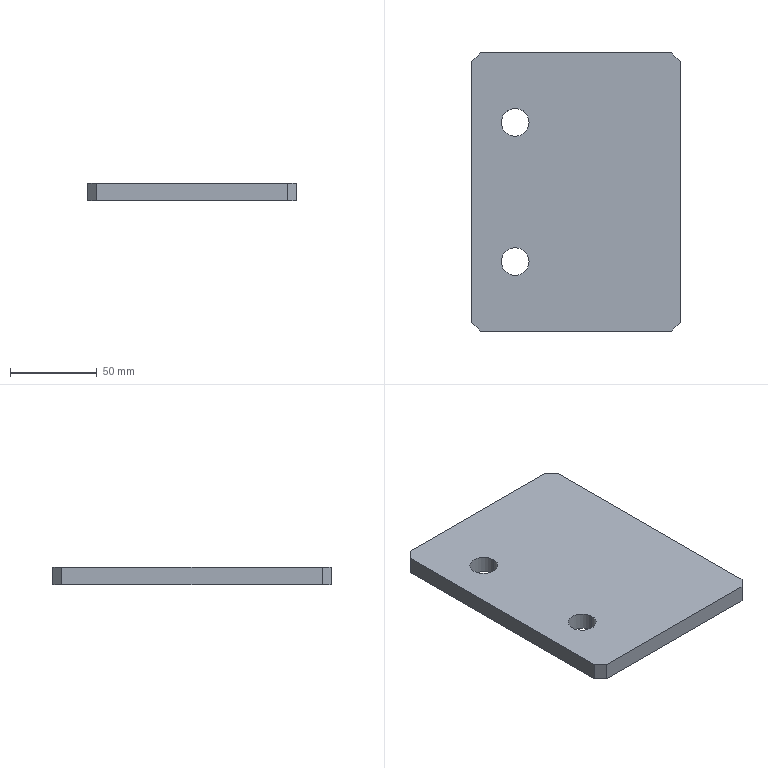Part | STEP file | 中转釜楼梯Pad 1 | 1 solid | 14 faces | box 120 x 160 x 10 mm | volume 187479 mm3 | plane 10 | cylinder 4 | commonest cylinder face diameters 16 x4
STEP:
#1=CARTESIAN_POINT('',(0.,0.,0.));
#2=DIRECTION('',(0.,0.,1.));
#3=DIRECTION('',(1.,0.,0.));
#4=AXIS2_PLACEMENT_3D('',#1,#2,#3);
#5=CARTESIAN_POINT('',(-27.,40.,0.));
#6=VERTEX_POINT('',#5);
#7=CARTESIAN_POINT('',(-27.,40.,10.));
#8=VERTEX_POINT('',#7);
#9=CARTESIAN_POINT('',(-27.,40.,10.));
#10=DIRECTION('',(0.,0.,1.));
#11=VECTOR('',#10,1.);
#12=LINE('',#9,#11);
#13=CARTESIAN_POINT('',(-35.,40.,10.));
#14=DIRECTION('',(0.,0.,1.));
#15=DIRECTION('',(1.,0.,0.));
#16=AXIS2_PLACEMENT_3D('',#13,#14,#15);
#17=CYLINDRICAL_SURFACE('',#16,8.);
#18=CARTESIAN_POINT('',(6.283,0.));
#19=DIRECTION('',(0.,1.));
#20=VECTOR('',#19,1.);
#21=LINE('',#18,#20);
#22=(GEOMETRIC_REPRESENTATION_CONTEXT(2)PARAMETRIC_REPRESENTATION_CONTEXT()REPRESENTATION_CONTEXT('',''));
#23=DEFINITIONAL_REPRESENTATION('',(#21),#22);
#24=PCURVE('',#17,#23);
#25=CARTESIAN_POINT('',(-35.,40.,10.));
#26=DIRECTION('',(0.,0.,1.));
#27=DIRECTION('',(1.,0.,0.));
#28=AXIS2_PLACEMENT_3D('',#25,#26,#27);
#29=CYLINDRICAL_SURFACE('',#28,8.);
#30=CARTESIAN_POINT('',(0.,0.));
#31=DIRECTION('',(0.,1.));
#32=VECTOR('',#31,1.);
#33=LINE('',#30,#32);
#34=(GEOMETRIC_REPRESENTATION_CONTEXT(2)PARAMETRIC_REPRESENTATION_CONTEXT()REPRESENTATION_CONTEXT('',''));
#35=DEFINITIONAL_REPRESENTATION('',(#33),#34);
#36=PCURVE('',#29,#35);
#37=SURFACE_CURVE('',#12,(#24,#36),.PCURVE_S1.);
#38=EDGE_CURVE('',#6,#8,#37,.T.);
#39=ORIENTED_EDGE('',*,*,#38,.T.);
#40=CARTESIAN_POINT('',(-43.,40.,10.));
#41=VERTEX_POINT('',#40);
#42=CARTESIAN_POINT('',(-35.,40.,10.));
#43=DIRECTION('',(0.,0.,1.));
#44=DIRECTION('',(1.,0.,0.));
#45=AXIS2_PLACEMENT_3D('',#42,#43,#44);
#46=CIRCLE('',#45,8.);
#47=CARTESIAN_POINT('',(0.,0.));
#48=DIRECTION('',(1.,0.));
#49=VECTOR('',#48,1.);
#50=LINE('',#47,#49);
#51=(GEOMETRIC_REPRESENTATION_CONTEXT(2)PARAMETRIC_REPRESENTATION_CONTEXT()REPRESENTATION_CONTEXT('',''));
#52=DEFINITIONAL_REPRESENTATION('',(#50),#51);
#53=PCURVE('',#17,#52);
#54=CARTESIAN_POINT('',(0.,0.,10.));
#55=DIRECTION('',(0.,0.,1.));
#56=DIRECTION('',(1.,0.,0.));
#57=AXIS2_PLACEMENT_3D('',#54,#55,#56);
#58=PLANE('',#57);
#59=CARTESIAN_POINT('',(-35.,40.));
#60=DIRECTION('',(1.,0.));
#61=AXIS2_PLACEMENT_2D('',#59,#60);
#62=CIRCLE('',#61,8.);
#63=(GEOMETRIC_REPRESENTATION_CONTEXT(2)PARAMETRIC_REPRESENTATION_CONTEXT()REPRESENTATION_CONTEXT('',''));
#64=DEFINITIONAL_REPRESENTATION('',(#62),#63);
#65=PCURVE('',#58,#64);
#66=SURFACE_CURVE('',#46,(#53,#65),.PCURVE_S1.);
#67=EDGE_CURVE('',#41,#8,#66,.T.);
#68=ORIENTED_EDGE('',*,*,#67,.F.);
#69=CARTESIAN_POINT('',(-43.,40.,0.));
#70=VERTEX_POINT('',#69);
#71=CARTESIAN_POINT('',(-43.,40.,10.));
#72=DIRECTION('',(0.,0.,1.));
#73=VECTOR('',#72,1.);
#74=LINE('',#71,#73);
#75=CARTESIAN_POINT('',(3.142,0.));
#76=DIRECTION('',(0.,1.));
#77=VECTOR('',#76,1.);
#78=LINE('',#75,#77);
#79=(GEOMETRIC_REPRESENTATION_CONTEXT(2)PARAMETRIC_REPRESENTATION_CONTEXT()REPRESENTATION_CONTEXT('',''));
#80=DEFINITIONAL_REPRESENTATION('',(#78),#79);
#81=PCURVE('',#17,#80);
#82=CARTESIAN_POINT('',(3.142,0.));
#83=DIRECTION('',(0.,1.));
#84=VECTOR('',#83,1.);
#85=LINE('',#82,#84);
#86=(GEOMETRIC_REPRESENTATION_CONTEXT(2)PARAMETRIC_REPRESENTATION_CONTEXT()REPRESENTATION_CONTEXT('',''));
#87=DEFINITIONAL_REPRESENTATION('',(#85),#86);
#88=PCURVE('',#29,#87);
#89=SURFACE_CURVE('',#74,(#81,#88),.PCURVE_S1.);
#90=EDGE_CURVE('',#70,#41,#89,.T.);
#91=ORIENTED_EDGE('',*,*,#90,.F.);
#92=CARTESIAN_POINT('',(-35.,40.,0.));
#93=DIRECTION('',(0.,0.,1.));
#94=DIRECTION('',(1.,0.,0.));
#95=AXIS2_PLACEMENT_3D('',#92,#93,#94);
#96=CIRCLE('',#95,8.);
#97=CARTESIAN_POINT('',(0.,-10.));
#98=DIRECTION('',(1.,0.));
#99=VECTOR('',#98,1.);
#100=LINE('',#97,#99);
#101=(GEOMETRIC_REPRESENTATION_CONTEXT(2)PARAMETRIC_REPRESENTATION_CONTEXT()REPRESENTATION_CONTEXT('',''));
#102=DEFINITIONAL_REPRESENTATION('',(#100),#101);
#103=PCURVE('',#17,#102);
#104=CARTESIAN_POINT('',(0.,0.,0.));
#105=DIRECTION('',(0.,0.,1.));
#106=DIRECTION('',(1.,0.,0.));
#107=AXIS2_PLACEMENT_3D('',#104,#105,#106);
#108=PLANE('',#107);
#109=CARTESIAN_POINT('',(-35.,40.));
#110=DIRECTION('',(1.,0.));
#111=AXIS2_PLACEMENT_2D('',#109,#110);
#112=CIRCLE('',#111,8.);
#113=(GEOMETRIC_REPRESENTATION_CONTEXT(2)PARAMETRIC_REPRESENTATION_CONTEXT()REPRESENTATION_CONTEXT('',''));
#114=DEFINITIONAL_REPRESENTATION('',(#112),#113);
#115=PCURVE('',#108,#114);
#116=SURFACE_CURVE('',#96,(#103,#115),.PCURVE_S1.);
#117=EDGE_CURVE('',#70,#6,#116,.T.);
#118=ORIENTED_EDGE('',*,*,#117,.T.);
#119=EDGE_LOOP('',(#39,#68,#91,#118));
#120=FACE_BOUND('',#119,.F.);
#121=ADVANCED_FACE('',(#120),#17,.F.);
#122=CARTESIAN_POINT('',(-27.,120.,0.));
#123=VERTEX_POINT('',#122);
#124=CARTESIAN_POINT('',(-27.,120.,10.));
#125=VERTEX_POINT('',#124);
#126=CARTESIAN_POINT('',(-27.,120.,10.));
#127=DIRECTION('',(0.,0.,1.));
#128=VECTOR('',#127,1.);
#129=LINE('',#126,#128);
#130=CARTESIAN_POINT('',(-35.,120.,10.));
#131=DIRECTION('',(0.,0.,1.));
#132=DIRECTION('',(1.,0.,0.));
#133=AXIS2_PLACEMENT_3D('',#130,#131,#132);
#134=CYLINDRICAL_SURFACE('',#133,8.);
#135=CARTESIAN_POINT('',(6.283,0.));
#136=DIRECTION('',(0.,1.));
#137=VECTOR('',#136,1.);
#138=LINE('',#135,#137);
#139=(GEOMETRIC_REPRESENTATION_CONTEXT(2)PARAMETRIC_REPRESENTATION_CONTEXT()REPRESENTATION_CONTEXT('',''));
#140=DEFINITIONAL_REPRESENTATION('',(#138),#139);
#141=PCURVE('',#134,#140);
#142=CARTESIAN_POINT('',(-35.,120.,10.));
#143=DIRECTION('',(0.,0.,1.));
#144=DIRECTION('',(1.,0.,0.));
#145=AXIS2_PLACEMENT_3D('',#142,#143,#144);
#146=CYLINDRICAL_SURFACE('',#145,8.);
#147=CARTESIAN_POINT('',(0.,0.));
#148=DIRECTION('',(0.,1.));
#149=VECTOR('',#148,1.);
#150=LINE('',#147,#149);
#151=(GEOMETRIC_REPRESENTATION_CONTEXT(2)PARAMETRIC_REPRESENTATION_CONTEXT()REPRESENTATION_CONTEXT('',''));
#152=DEFINITIONAL_REPRESENTATION('',(#150),#151);
#153=PCURVE('',#146,#152);
#154=SURFACE_CURVE('',#129,(#141,#153),.PCURVE_S1.);
#155=EDGE_CURVE('',#123,#125,#154,.T.);
#156=ORIENTED_EDGE('',*,*,#155,.T.);
#157=CARTESIAN_POINT('',(-43.,120.,10.));
#158=VERTEX_POINT('',#157);
#159=CARTESIAN_POINT('',(-35.,120.,10.));
#160=DIRECTION('',(0.,0.,1.));
#161=DIRECTION('',(1.,0.,0.));
#162=AXIS2_PLACEMENT_3D('',#159,#160,#161);
#163=CIRCLE('',#162,8.);
#164=CARTESIAN_POINT('',(0.,0.));
#165=DIRECTION('',(1.,0.));
#166=VECTOR('',#165,1.);
#167=LINE('',#164,#166);
#168=(GEOMETRIC_REPRESENTATION_CONTEXT(2)PARAMETRIC_REPRESENTATION_CONTEXT()REPRESENTATION_CONTEXT('',''));
#169=DEFINITIONAL_REPRESENTATION('',(#167),#168);
#170=PCURVE('',#134,#169);
#171=CARTESIAN_POINT('',(-35.,120.));
#172=DIRECTION('',(1.,0.));
#173=AXIS2_PLACEMENT_2D('',#171,#172);
#174=CIRCLE('',#173,8.);
#175=(GEOMETRIC_REPRESENTATION_CONTEXT(2)PARAMETRIC_REPRESENTATION_CONTEXT()REPRESENTATION_CONTEXT('',''));
#176=DEFINITIONAL_REPRESENTATION('',(#174),#175);
#177=PCURVE('',#58,#176);
#178=SURFACE_CURVE('',#163,(#170,#177),.PCURVE_S1.);
#179=EDGE_CURVE('',#158,#125,#178,.T.);
#180=ORIENTED_EDGE('',*,*,#179,.F.);
#181=CARTESIAN_POINT('',(-43.,120.,0.));
#182=VERTEX_POINT('',#181);
#183=CARTESIAN_POINT('',(-43.,120.,10.));
#184=DIRECTION('',(0.,0.,1.));
#185=VECTOR('',#184,1.);
#186=LINE('',#183,#185);
#187=CARTESIAN_POINT('',(3.142,0.));
#188=DIRECTION('',(0.,1.));
#189=VECTOR('',#188,1.);
#190=LINE('',#187,#189);
#191=(GEOMETRIC_REPRESENTATION_CONTEXT(2)PARAMETRIC_REPRESENTATION_CONTEXT()REPRESENTATION_CONTEXT('',''));
#192=DEFINITIONAL_REPRESENTATION('',(#190),#191);
#193=PCURVE('',#134,#192);
#194=CARTESIAN_POINT('',(3.142,0.));
#195=DIRECTION('',(0.,1.));
#196=VECTOR('',#195,1.);
#197=LINE('',#194,#196);
#198=(GEOMETRIC_REPRESENTATION_CONTEXT(2)PARAMETRIC_REPRESENTATION_CONTEXT()REPRESENTATION_CONTEXT('',''));
#199=DEFINITIONAL_REPRESENTATION('',(#197),#198);
#200=PCURVE('',#146,#199);
#201=SURFACE_CURVE('',#186,(#193,#200),.PCURVE_S1.);
#202=EDGE_CURVE('',#182,#158,#201,.T.);
#203=ORIENTED_EDGE('',*,*,#202,.F.);
#204=CARTESIAN_POINT('',(-35.,120.,0.));
#205=DIRECTION('',(0.,0.,1.));
#206=DIRECTION('',(1.,0.,0.));
#207=AXIS2_PLACEMENT_3D('',#204,#205,#206);
#208=CIRCLE('',#207,8.);
#209=CARTESIAN_POINT('',(0.,-10.));
#210=DIRECTION('',(1.,0.));
#211=VECTOR('',#210,1.);
#212=LINE('',#209,#211);
#213=(GEOMETRIC_REPRESENTATION_CONTEXT(2)PARAMETRIC_REPRESENTATION_CONTEXT()REPRESENTATION_CONTEXT('',''));
#214=DEFINITIONAL_REPRESENTATION('',(#212),#213);
#215=PCURVE('',#134,#214);
#216=CARTESIAN_POINT('',(-35.,120.));
#217=DIRECTION('',(1.,0.));
#218=AXIS2_PLACEMENT_2D('',#216,#217);
#219=CIRCLE('',#218,8.);
#220=(GEOMETRIC_REPRESENTATION_CONTEXT(2)PARAMETRIC_REPRESENTATION_CONTEXT()REPRESENTATION_CONTEXT('',''));
#221=DEFINITIONAL_REPRESENTATION('',(#219),#220);
#222=PCURVE('',#108,#221);
#223=SURFACE_CURVE('',#208,(#215,#222),.PCURVE_S1.);
#224=EDGE_CURVE('',#182,#123,#223,.T.);
#225=ORIENTED_EDGE('',*,*,#224,.T.);
#226=EDGE_LOOP('',(#156,#180,#203,#225));
#227=FACE_BOUND('',#226,.F.);
#228=ADVANCED_FACE('',(#227),#134,.F.);
#229=CARTESIAN_POINT('',(-60.,155.,0.));
#230=VERTEX_POINT('',#229);
#231=CARTESIAN_POINT('',(-60.,5.,0.));
#232=VERTEX_POINT('',#231);
#233=CARTESIAN_POINT('',(-60.,160.,0.));
#234=DIRECTION('',(0.,-1.,0.));
#235=VECTOR('',#234,1.);
#236=LINE('',#233,#235);
#237=CARTESIAN_POINT('',(-60.,160.,10.));
#238=DIRECTION('',(1.,0.,0.));
#239=DIRECTION('',(0.,1.,0.));
#240=AXIS2_PLACEMENT_3D('',#237,#238,#239);
#241=PLANE('',#240);
#242=CARTESIAN_POINT('',(0.,-10.));
#243=DIRECTION('',(-1.,0.));
#244=VECTOR('',#243,1.);
#245=LINE('',#242,#244);
#246=(GEOMETRIC_REPRESENTATION_CONTEXT(2)PARAMETRIC_REPRESENTATION_CONTEXT()REPRESENTATION_CONTEXT('',''));
#247=DEFINITIONAL_REPRESENTATION('',(#245),#246);
#248=PCURVE('',#241,#247);
#249=CARTESIAN_POINT('',(-60.,160.));
#250=DIRECTION('',(0.,-1.));
#251=VECTOR('',#250,1.);
#252=LINE('',#249,#251);
#253=(GEOMETRIC_REPRESENTATION_CONTEXT(2)PARAMETRIC_REPRESENTATION_CONTEXT()REPRESENTATION_CONTEXT('',''));
#254=DEFINITIONAL_REPRESENTATION('',(#252),#253);
#255=PCURVE('',#108,#254);
#256=SURFACE_CURVE('',#236,(#248,#255),.PCURVE_S1.);
#257=EDGE_CURVE('',#230,#232,#256,.T.);
#258=ORIENTED_EDGE('',*,*,#257,.T.);
#259=CARTESIAN_POINT('',(-60.,5.,10.));
#260=VERTEX_POINT('',#259);
#261=CARTESIAN_POINT('',(-60.,5.,10.));
#262=DIRECTION('',(0.,0.,1.));
#263=VECTOR('',#262,1.);
#264=LINE('',#261,#263);
#265=CARTESIAN_POINT('',(-155.,0.));
#266=DIRECTION('',(0.,1.));
#267=VECTOR('',#266,1.);
#268=LINE('',#265,#267);
#269=(GEOMETRIC_REPRESENTATION_CONTEXT(2)PARAMETRIC_REPRESENTATION_CONTEXT()REPRESENTATION_CONTEXT('',''));
#270=DEFINITIONAL_REPRESENTATION('',(#268),#269);
#271=PCURVE('',#241,#270);
#272=CARTESIAN_POINT('',(-55.,0.,10.));
#273=DIRECTION('',(0.7071,0.7071,0.));
#274=DIRECTION('',(0.,0.,-1.));
#275=AXIS2_PLACEMENT_3D('',#272,#273,#274);
#276=PLANE('',#275);
#277=CARTESIAN_POINT('',(0.,7.071));
#278=DIRECTION('',(-1.,0.));
#279=VECTOR('',#278,1.);
#280=LINE('',#277,#279);
#281=(GEOMETRIC_REPRESENTATION_CONTEXT(2)PARAMETRIC_REPRESENTATION_CONTEXT()REPRESENTATION_CONTEXT('',''));
#282=DEFINITIONAL_REPRESENTATION('',(#280),#281);
#283=PCURVE('',#276,#282);
#284=SURFACE_CURVE('',#264,(#271,#283),.PCURVE_S1.);
#285=EDGE_CURVE('',#232,#260,#284,.T.);
#286=ORIENTED_EDGE('',*,*,#285,.T.);
#287=CARTESIAN_POINT('',(-60.,155.,10.));
#288=VERTEX_POINT('',#287);
#289=CARTESIAN_POINT('',(-60.,160.,10.));
#290=DIRECTION('',(0.,-1.,0.));
#291=VECTOR('',#290,1.);
#292=LINE('',#289,#291);
#293=CARTESIAN_POINT('',(0.,0.));
#294=DIRECTION('',(-1.,0.));
#295=VECTOR('',#294,1.);
#296=LINE('',#293,#295);
#297=(GEOMETRIC_REPRESENTATION_CONTEXT(2)PARAMETRIC_REPRESENTATION_CONTEXT()REPRESENTATION_CONTEXT('',''));
#298=DEFINITIONAL_REPRESENTATION('',(#296),#297);
#299=PCURVE('',#241,#298);
#300=CARTESIAN_POINT('',(-60.,160.));
#301=DIRECTION('',(0.,-1.));
#302=VECTOR('',#301,1.);
#303=LINE('',#300,#302);
#304=(GEOMETRIC_REPRESENTATION_CONTEXT(2)PARAMETRIC_REPRESENTATION_CONTEXT()REPRESENTATION_CONTEXT('',''));
#305=DEFINITIONAL_REPRESENTATION('',(#303),#304);
#306=PCURVE('',#58,#305);
#307=SURFACE_CURVE('',#292,(#299,#306),.PCURVE_S1.);
#308=EDGE_CURVE('',#288,#260,#307,.T.);
#309=ORIENTED_EDGE('',*,*,#308,.F.);
#310=CARTESIAN_POINT('',(-60.,155.,10.));
#311=DIRECTION('',(0.,0.,-1.));
#312=VECTOR('',#311,1.);
#313=LINE('',#310,#312);
#314=CARTESIAN_POINT('',(-5.,0.));
#315=DIRECTION('',(0.,-1.));
#316=VECTOR('',#315,1.);
#317=LINE('',#314,#316);
#318=(GEOMETRIC_REPRESENTATION_CONTEXT(2)PARAMETRIC_REPRESENTATION_CONTEXT()REPRESENTATION_CONTEXT('',''));
#319=DEFINITIONAL_REPRESENTATION('',(#317),#318);
#320=PCURVE('',#241,#319);
#321=CARTESIAN_POINT('',(-60.,155.,10.));
#322=DIRECTION('',(0.7071,-0.7071,0.));
#323=DIRECTION('',(0.,0.,-1.));
#324=AXIS2_PLACEMENT_3D('',#321,#322,#323);
#325=PLANE('',#324);
#326=CARTESIAN_POINT('',(0.,0.));
#327=DIRECTION('',(1.,0.));
#328=VECTOR('',#327,1.);
#329=LINE('',#326,#328);
#330=(GEOMETRIC_REPRESENTATION_CONTEXT(2)PARAMETRIC_REPRESENTATION_CONTEXT()REPRESENTATION_CONTEXT('',''));
#331=DEFINITIONAL_REPRESENTATION('',(#329),#330);
#332=PCURVE('',#325,#331);
#333=SURFACE_CURVE('',#313,(#320,#332),.PCURVE_S1.);
#334=EDGE_CURVE('',#288,#230,#333,.T.);
#335=ORIENTED_EDGE('',*,*,#334,.T.);
#336=EDGE_LOOP('',(#258,#286,#309,#335));
#337=FACE_BOUND('',#336,.T.);
#338=ADVANCED_FACE('',(#337),#241,.F.);
#339=CARTESIAN_POINT('',(-55.,0.,10.));
#340=VERTEX_POINT('',#339);
#341=CARTESIAN_POINT('',(55.,0.,10.));
#342=VERTEX_POINT('',#341);
#343=CARTESIAN_POINT('',(-60.,0.,10.));
#344=DIRECTION('',(1.,0.,0.));
#345=VECTOR('',#344,1.);
#346=LINE('',#343,#345);
#347=CARTESIAN_POINT('',(-60.,0.,10.));
#348=DIRECTION('',(0.,1.,0.));
#349=DIRECTION('',(0.,0.,1.));
#350=AXIS2_PLACEMENT_3D('',#347,#348,#349);
#351=PLANE('',#350);
#352=CARTESIAN_POINT('',(0.,0.));
#353=DIRECTION('',(0.,1.));
#354=VECTOR('',#353,1.);
#355=LINE('',#352,#354);
#356=(GEOMETRIC_REPRESENTATION_CONTEXT(2)PARAMETRIC_REPRESENTATION_CONTEXT()REPRESENTATION_CONTEXT('',''));
#357=DEFINITIONAL_REPRESENTATION('',(#355),#356);
#358=PCURVE('',#351,#357);
#359=CARTESIAN_POINT('',(-60.,0.));
#360=DIRECTION('',(1.,0.));
#361=VECTOR('',#360,1.);
#362=LINE('',#359,#361);
#363=(GEOMETRIC_REPRESENTATION_CONTEXT(2)PARAMETRIC_REPRESENTATION_CONTEXT()REPRESENTATION_CONTEXT('',''));
#364=DEFINITIONAL_REPRESENTATION('',(#362),#363);
#365=PCURVE('',#58,#364);
#366=SURFACE_CURVE('',#346,(#358,#365),.PCURVE_S1.);
#367=EDGE_CURVE('',#340,#342,#366,.T.);
#368=ORIENTED_EDGE('',*,*,#367,.F.);
#369=CARTESIAN_POINT('',(-55.,0.,0.));
#370=VERTEX_POINT('',#369);
#371=CARTESIAN_POINT('',(-55.,0.,10.));
#372=DIRECTION('',(0.,0.,-1.));
#373=VECTOR('',#372,1.);
#374=LINE('',#371,#373);
#375=CARTESIAN_POINT('',(0.,5.));
#376=DIRECTION('',(-1.,0.));
#377=VECTOR('',#376,1.);
#378=LINE('',#375,#377);
#379=(GEOMETRIC_REPRESENTATION_CONTEXT(2)PARAMETRIC_REPRESENTATION_CONTEXT()REPRESENTATION_CONTEXT('',''));
#380=DEFINITIONAL_REPRESENTATION('',(#378),#379);
#381=PCURVE('',#351,#380);
#382=CARTESIAN_POINT('',(0.,0.));
#383=DIRECTION('',(1.,0.));
#384=VECTOR('',#383,1.);
#385=LINE('',#382,#384);
#386=(GEOMETRIC_REPRESENTATION_CONTEXT(2)PARAMETRIC_REPRESENTATION_CONTEXT()REPRESENTATION_CONTEXT('',''));
#387=DEFINITIONAL_REPRESENTATION('',(#385),#386);
#388=PCURVE('',#276,#387);
#389=SURFACE_CURVE('',#374,(#381,#388),.PCURVE_S1.);
#390=EDGE_CURVE('',#340,#370,#389,.T.);
#391=ORIENTED_EDGE('',*,*,#390,.T.);
#392=CARTESIAN_POINT('',(55.,0.,0.));
#393=VERTEX_POINT('',#392);
#394=CARTESIAN_POINT('',(-60.,0.,0.));
#395=DIRECTION('',(1.,0.,0.));
#396=VECTOR('',#395,1.);
#397=LINE('',#394,#396);
#398=CARTESIAN_POINT('',(-10.,0.));
#399=DIRECTION('',(0.,1.));
#400=VECTOR('',#399,1.);
#401=LINE('',#398,#400);
#402=(GEOMETRIC_REPRESENTATION_CONTEXT(2)PARAMETRIC_REPRESENTATION_CONTEXT()REPRESENTATION_CONTEXT('',''));
#403=DEFINITIONAL_REPRESENTATION('',(#401),#402);
#404=PCURVE('',#351,#403);
#405=CARTESIAN_POINT('',(-60.,0.));
#406=DIRECTION('',(1.,0.));
#407=VECTOR('',#406,1.);
#408=LINE('',#405,#407);
#409=(GEOMETRIC_REPRESENTATION_CONTEXT(2)PARAMETRIC_REPRESENTATION_CONTEXT()REPRESENTATION_CONTEXT('',''));
#410=DEFINITIONAL_REPRESENTATION('',(#408),#409);
#411=PCURVE('',#108,#410);
#412=SURFACE_CURVE('',#397,(#404,#411),.PCURVE_S1.);
#413=EDGE_CURVE('',#370,#393,#412,.T.);
#414=ORIENTED_EDGE('',*,*,#413,.T.);
#415=CARTESIAN_POINT('',(55.,0.,10.));
#416=DIRECTION('',(0.,0.,1.));
#417=VECTOR('',#416,1.);
#418=LINE('',#415,#417);
#419=CARTESIAN_POINT('',(0.,115.));
#420=DIRECTION('',(1.,0.));
#421=VECTOR('',#420,1.);
#422=LINE('',#419,#421);
#423=(GEOMETRIC_REPRESENTATION_CONTEXT(2)PARAMETRIC_REPRESENTATION_CONTEXT()REPRESENTATION_CONTEXT('',''));
#424=DEFINITIONAL_REPRESENTATION('',(#422),#423);
#425=PCURVE('',#351,#424);
#426=CARTESIAN_POINT('',(60.,5.,10.));
#427=DIRECTION('',(-0.7071,0.7071,0.));
#428=DIRECTION('',(0.,0.,-1.));
#429=AXIS2_PLACEMENT_3D('',#426,#427,#428);
#430=PLANE('',#429);
#431=CARTESIAN_POINT('',(0.,7.071));
#432=DIRECTION('',(-1.,0.));
#433=VECTOR('',#432,1.);
#434=LINE('',#431,#433);
#435=(GEOMETRIC_REPRESENTATION_CONTEXT(2)PARAMETRIC_REPRESENTATION_CONTEXT()REPRESENTATION_CONTEXT('',''));
#436=DEFINITIONAL_REPRESENTATION('',(#434),#435);
#437=PCURVE('',#430,#436);
#438=SURFACE_CURVE('',#418,(#425,#437),.PCURVE_S1.);
#439=EDGE_CURVE('',#393,#342,#438,.T.);
#440=ORIENTED_EDGE('',*,*,#439,.T.);
#441=EDGE_LOOP('',(#368,#391,#414,#440));
#442=FACE_BOUND('',#441,.T.);
#443=ADVANCED_FACE('',(#442),#351,.F.);
#444=CARTESIAN_POINT('',(60.,5.,10.));
#445=VERTEX_POINT('',#444);
#446=CARTESIAN_POINT('',(60.,155.,10.));
#447=VERTEX_POINT('',#446);
#448=CARTESIAN_POINT('',(60.,160.,10.));
#449=DIRECTION('',(0.,1.,0.));
#450=VECTOR('',#449,1.);
#451=LINE('',#448,#450);
#452=CARTESIAN_POINT('',(60.,160.,10.));
#453=DIRECTION('',(-1.,0.,0.));
#454=DIRECTION('',(0.,-1.,0.));
#455=AXIS2_PLACEMENT_3D('',#452,#453,#454);
#456=PLANE('',#455);
#457=CARTESIAN_POINT('',(0.,0.));
#458=DIRECTION('',(-1.,0.));
#459=VECTOR('',#458,1.);
#460=LINE('',#457,#459);
#461=(GEOMETRIC_REPRESENTATION_CONTEXT(2)PARAMETRIC_REPRESENTATION_CONTEXT()REPRESENTATION_CONTEXT('',''));
#462=DEFINITIONAL_REPRESENTATION('',(#460),#461);
#463=PCURVE('',#456,#462);
#464=CARTESIAN_POINT('',(60.,160.));
#465=DIRECTION('',(0.,1.));
#466=VECTOR('',#465,1.);
#467=LINE('',#464,#466);
#468=(GEOMETRIC_REPRESENTATION_CONTEXT(2)PARAMETRIC_REPRESENTATION_CONTEXT()REPRESENTATION_CONTEXT('',''));
#469=DEFINITIONAL_REPRESENTATION('',(#467),#468);
#470=PCURVE('',#58,#469);
#471=SURFACE_CURVE('',#451,(#463,#470),.PCURVE_S1.);
#472=EDGE_CURVE('',#445,#447,#471,.T.);
#473=ORIENTED_EDGE('',*,*,#472,.F.);
#474=CARTESIAN_POINT('',(60.,5.,0.));
#475=VERTEX_POINT('',#474);
#476=CARTESIAN_POINT('',(60.,5.,10.));
#477=DIRECTION('',(0.,0.,-1.));
#478=VECTOR('',#477,1.);
#479=LINE('',#476,#478);
#480=CARTESIAN_POINT('',(155.,0.));
#481=DIRECTION('',(0.,-1.));
#482=VECTOR('',#481,1.);
#483=LINE('',#480,#482);
#484=(GEOMETRIC_REPRESENTATION_CONTEXT(2)PARAMETRIC_REPRESENTATION_CONTEXT()REPRESENTATION_CONTEXT('',''));
#485=DEFINITIONAL_REPRESENTATION('',(#483),#484);
#486=PCURVE('',#456,#485);
#487=CARTESIAN_POINT('',(0.,0.));
#488=DIRECTION('',(1.,0.));
#489=VECTOR('',#488,1.);
#490=LINE('',#487,#489);
#491=(GEOMETRIC_REPRESENTATION_CONTEXT(2)PARAMETRIC_REPRESENTATION_CONTEXT()REPRESENTATION_CONTEXT('',''));
#492=DEFINITIONAL_REPRESENTATION('',(#490),#491);
#493=PCURVE('',#430,#492);
#494=SURFACE_CURVE('',#479,(#486,#493),.PCURVE_S1.);
#495=EDGE_CURVE('',#445,#475,#494,.T.);
#496=ORIENTED_EDGE('',*,*,#495,.T.);
#497=CARTESIAN_POINT('',(60.,155.,0.));
#498=VERTEX_POINT('',#497);
#499=CARTESIAN_POINT('',(60.,160.,0.));
#500=DIRECTION('',(0.,1.,0.));
#501=VECTOR('',#500,1.);
#502=LINE('',#499,#501);
#503=CARTESIAN_POINT('',(0.,-10.));
#504=DIRECTION('',(-1.,0.));
#505=VECTOR('',#504,1.);
#506=LINE('',#503,#505);
#507=(GEOMETRIC_REPRESENTATION_CONTEXT(2)PARAMETRIC_REPRESENTATION_CONTEXT()REPRESENTATION_CONTEXT('',''));
#508=DEFINITIONAL_REPRESENTATION('',(#506),#507);
#509=PCURVE('',#456,#508);
#510=CARTESIAN_POINT('',(60.,160.));
#511=DIRECTION('',(0.,1.));
#512=VECTOR('',#511,1.);
#513=LINE('',#510,#512);
#514=(GEOMETRIC_REPRESENTATION_CONTEXT(2)PARAMETRIC_REPRESENTATION_CONTEXT()REPRESENTATION_CONTEXT('',''));
#515=DEFINITIONAL_REPRESENTATION('',(#513),#514);
#516=PCURVE('',#108,#515);
#517=SURFACE_CURVE('',#502,(#509,#516),.PCURVE_S1.);
#518=EDGE_CURVE('',#475,#498,#517,.T.);
#519=ORIENTED_EDGE('',*,*,#518,.T.);
#520=CARTESIAN_POINT('',(60.,155.,10.));
#521=DIRECTION('',(0.,0.,1.));
#522=VECTOR('',#521,1.);
#523=LINE('',#520,#522);
#524=CARTESIAN_POINT('',(5.,0.));
#525=DIRECTION('',(0.,1.));
#526=VECTOR('',#525,1.);
#527=LINE('',#524,#526);
#528=(GEOMETRIC_REPRESENTATION_CONTEXT(2)PARAMETRIC_REPRESENTATION_CONTEXT()REPRESENTATION_CONTEXT('',''));
#529=DEFINITIONAL_REPRESENTATION('',(#527),#528);
#530=PCURVE('',#456,#529);
#531=CARTESIAN_POINT('',(55.,160.,10.));
#532=DIRECTION('',(-0.7071,-0.7071,0.));
#533=DIRECTION('',(0.,0.,-1.));
#534=AXIS2_PLACEMENT_3D('',#531,#532,#533);
#535=PLANE('',#534);
#536=CARTESIAN_POINT('',(0.,7.071));
#537=DIRECTION('',(-1.,0.));
#538=VECTOR('',#537,1.);
#539=LINE('',#536,#538);
#540=(GEOMETRIC_REPRESENTATION_CONTEXT(2)PARAMETRIC_REPRESENTATION_CONTEXT()REPRESENTATION_CONTEXT('',''));
#541=DEFINITIONAL_REPRESENTATION('',(#539),#540);
#542=PCURVE('',#535,#541);
#543=SURFACE_CURVE('',#523,(#530,#542),.PCURVE_S1.);
#544=EDGE_CURVE('',#498,#447,#543,.T.);
#545=ORIENTED_EDGE('',*,*,#544,.T.);
#546=EDGE_LOOP('',(#473,#496,#519,#545));
#547=FACE_BOUND('',#546,.T.);
#548=ADVANCED_FACE('',(#547),#456,.F.);
#549=CARTESIAN_POINT('',(55.,160.,10.));
#550=VERTEX_POINT('',#549);
#551=CARTESIAN_POINT('',(-55.,160.,10.));
#552=VERTEX_POINT('',#551);
#553=CARTESIAN_POINT('',(-60.,160.,10.));
#554=DIRECTION('',(-1.,0.,0.));
#555=VECTOR('',#554,1.);
#556=LINE('',#553,#555);
#557=CARTESIAN_POINT('',(-60.,160.,10.));
#558=DIRECTION('',(0.,-1.,0.));
#559=DIRECTION('',(0.,0.,-1.));
#560=AXIS2_PLACEMENT_3D('',#557,#558,#559);
#561=PLANE('',#560);
#562=CARTESIAN_POINT('',(0.,0.));
#563=DIRECTION('',(0.,-1.));
#564=VECTOR('',#563,1.);
#565=LINE('',#562,#564);
#566=(GEOMETRIC_REPRESENTATION_CONTEXT(2)PARAMETRIC_REPRESENTATION_CONTEXT()REPRESENTATION_CONTEXT('',''));
#567=DEFINITIONAL_REPRESENTATION('',(#565),#566);
#568=PCURVE('',#561,#567);
#569=CARTESIAN_POINT('',(-60.,160.));
#570=DIRECTION('',(-1.,0.));
#571=VECTOR('',#570,1.);
#572=LINE('',#569,#571);
#573=(GEOMETRIC_REPRESENTATION_CONTEXT(2)PARAMETRIC_REPRESENTATION_CONTEXT()REPRESENTATION_CONTEXT('',''));
#574=DEFINITIONAL_REPRESENTATION('',(#572),#573);
#575=PCURVE('',#58,#574);
#576=SURFACE_CURVE('',#556,(#568,#575),.PCURVE_S1.);
#577=EDGE_CURVE('',#550,#552,#576,.T.);
#578=ORIENTED_EDGE('',*,*,#577,.F.);
#579=CARTESIAN_POINT('',(55.,160.,0.));
#580=VERTEX_POINT('',#579);
#581=CARTESIAN_POINT('',(55.,160.,10.));
#582=DIRECTION('',(0.,0.,-1.));
#583=VECTOR('',#582,1.);
#584=LINE('',#581,#583);
#585=CARTESIAN_POINT('',(0.,115.));
#586=DIRECTION('',(1.,0.));
#587=VECTOR('',#586,1.);
#588=LINE('',#585,#587);
#589=(GEOMETRIC_REPRESENTATION_CONTEXT(2)PARAMETRIC_REPRESENTATION_CONTEXT()REPRESENTATION_CONTEXT('',''));
#590=DEFINITIONAL_REPRESENTATION('',(#588),#589);
#591=PCURVE('',#561,#590);
#592=CARTESIAN_POINT('',(0.,0.));
#593=DIRECTION('',(1.,0.));
#594=VECTOR('',#593,1.);
#595=LINE('',#592,#594);
#596=(GEOMETRIC_REPRESENTATION_CONTEXT(2)PARAMETRIC_REPRESENTATION_CONTEXT()REPRESENTATION_CONTEXT('',''));
#597=DEFINITIONAL_REPRESENTATION('',(#595),#596);
#598=PCURVE('',#535,#597);
#599=SURFACE_CURVE('',#584,(#591,#598),.PCURVE_S1.);
#600=EDGE_CURVE('',#550,#580,#599,.T.);
#601=ORIENTED_EDGE('',*,*,#600,.T.);
#602=CARTESIAN_POINT('',(-55.,160.,0.));
#603=VERTEX_POINT('',#602);
#604=CARTESIAN_POINT('',(-60.,160.,0.));
#605=DIRECTION('',(-1.,0.,0.));
#606=VECTOR('',#605,1.);
#607=LINE('',#604,#606);
#608=CARTESIAN_POINT('',(10.,0.));
#609=DIRECTION('',(0.,-1.));
#610=VECTOR('',#609,1.);
#611=LINE('',#608,#610);
#612=(GEOMETRIC_REPRESENTATION_CONTEXT(2)PARAMETRIC_REPRESENTATION_CONTEXT()REPRESENTATION_CONTEXT('',''));
#613=DEFINITIONAL_REPRESENTATION('',(#611),#612);
#614=PCURVE('',#561,#613);
#615=CARTESIAN_POINT('',(-60.,160.));
#616=DIRECTION('',(-1.,0.));
#617=VECTOR('',#616,1.);
#618=LINE('',#615,#617);
#619=(GEOMETRIC_REPRESENTATION_CONTEXT(2)PARAMETRIC_REPRESENTATION_CONTEXT()REPRESENTATION_CONTEXT('',''));
#620=DEFINITIONAL_REPRESENTATION('',(#618),#619);
#621=PCURVE('',#108,#620);
#622=SURFACE_CURVE('',#607,(#614,#621),.PCURVE_S1.);
#623=EDGE_CURVE('',#580,#603,#622,.T.);
#624=ORIENTED_EDGE('',*,*,#623,.T.);
#625=CARTESIAN_POINT('',(-55.,160.,10.));
#626=DIRECTION('',(0.,0.,1.));
#627=VECTOR('',#626,1.);
#628=LINE('',#625,#627);
#629=CARTESIAN_POINT('',(0.,5.));
#630=DIRECTION('',(-1.,0.));
#631=VECTOR('',#630,1.);
#632=LINE('',#629,#631);
#633=(GEOMETRIC_REPRESENTATION_CONTEXT(2)PARAMETRIC_REPRESENTATION_CONTEXT()REPRESENTATION_CONTEXT('',''));
#634=DEFINITIONAL_REPRESENTATION('',(#632),#633);
#635=PCURVE('',#561,#634);
#636=CARTESIAN_POINT('',(0.,7.071));
#637=DIRECTION('',(-1.,0.));
#638=VECTOR('',#637,1.);
#639=LINE('',#636,#638);
#640=(GEOMETRIC_REPRESENTATION_CONTEXT(2)PARAMETRIC_REPRESENTATION_CONTEXT()REPRESENTATION_CONTEXT('',''));
#641=DEFINITIONAL_REPRESENTATION('',(#639),#640);
#642=PCURVE('',#325,#641);
#643=SURFACE_CURVE('',#628,(#635,#642),.PCURVE_S1.);
#644=EDGE_CURVE('',#603,#552,#643,.T.);
#645=ORIENTED_EDGE('',*,*,#644,.T.);
#646=EDGE_LOOP('',(#578,#601,#624,#645));
#647=FACE_BOUND('',#646,.T.);
#648=ADVANCED_FACE('',(#647),#561,.F.);
#649=CARTESIAN_POINT('',(-35.,40.,10.));
#650=DIRECTION('',(0.,0.,1.));
#651=DIRECTION('',(1.,0.,0.));
#652=AXIS2_PLACEMENT_3D('',#649,#650,#651);
#653=CIRCLE('',#652,8.);
#654=CARTESIAN_POINT('',(-35.,40.));
#655=DIRECTION('',(1.,0.));
#656=AXIS2_PLACEMENT_2D('',#654,#655);
#657=CIRCLE('',#656,8.);
#658=(GEOMETRIC_REPRESENTATION_CONTEXT(2)PARAMETRIC_REPRESENTATION_CONTEXT()REPRESENTATION_CONTEXT('',''));
#659=DEFINITIONAL_REPRESENTATION('',(#657),#658);
#660=PCURVE('',#58,#659);
#661=CARTESIAN_POINT('',(0.,0.));
#662=DIRECTION('',(1.,0.));
#663=VECTOR('',#662,1.);
#664=LINE('',#661,#663);
#665=(GEOMETRIC_REPRESENTATION_CONTEXT(2)PARAMETRIC_REPRESENTATION_CONTEXT()REPRESENTATION_CONTEXT('',''));
#666=DEFINITIONAL_REPRESENTATION('',(#664),#665);
#667=PCURVE('',#29,#666);
#668=SURFACE_CURVE('',#653,(#660,#667),.PCURVE_S1.);
#669=EDGE_CURVE('',#8,#41,#668,.T.);
#670=ORIENTED_EDGE('',*,*,#669,.F.);
#671=ORIENTED_EDGE('',*,*,#67,.F.);
#672=EDGE_LOOP('',(#670,#671));
#673=FACE_BOUND('',#672,.T.);
#674=CARTESIAN_POINT('',(-35.,120.,10.));
#675=DIRECTION('',(0.,0.,1.));
#676=DIRECTION('',(1.,0.,0.));
#677=AXIS2_PLACEMENT_3D('',#674,#675,#676);
#678=CIRCLE('',#677,8.);
#679=CARTESIAN_POINT('',(-35.,120.));
#680=DIRECTION('',(1.,0.));
#681=AXIS2_PLACEMENT_2D('',#679,#680);
#682=CIRCLE('',#681,8.);
#683=(GEOMETRIC_REPRESENTATION_CONTEXT(2)PARAMETRIC_REPRESENTATION_CONTEXT()REPRESENTATION_CONTEXT('',''));
#684=DEFINITIONAL_REPRESENTATION('',(#682),#683);
#685=PCURVE('',#58,#684);
#686=CARTESIAN_POINT('',(0.,0.));
#687=DIRECTION('',(1.,0.));
#688=VECTOR('',#687,1.);
#689=LINE('',#686,#688);
#690=(GEOMETRIC_REPRESENTATION_CONTEXT(2)PARAMETRIC_REPRESENTATION_CONTEXT()REPRESENTATION_CONTEXT('',''));
#691=DEFINITIONAL_REPRESENTATION('',(#689),#690);
#692=PCURVE('',#146,#691);
#693=SURFACE_CURVE('',#678,(#685,#692),.PCURVE_S1.);
#694=EDGE_CURVE('',#125,#158,#693,.T.);
#695=ORIENTED_EDGE('',*,*,#694,.F.);
#696=ORIENTED_EDGE('',*,*,#179,.F.);
#697=EDGE_LOOP('',(#695,#696));
#698=FACE_BOUND('',#697,.T.);
#699=ORIENTED_EDGE('',*,*,#308,.T.);
#700=CARTESIAN_POINT('',(-27.5,-27.5,10.));
#701=DIRECTION('',(0.7071,-0.7071,0.));
#702=VECTOR('',#701,1.);
#703=LINE('',#700,#702);
#704=CARTESIAN_POINT('',(-27.5,-27.5));
#705=DIRECTION('',(0.7071,-0.7071));
#706=VECTOR('',#705,1.);
#707=LINE('',#704,#706);
#708=(GEOMETRIC_REPRESENTATION_CONTEXT(2)PARAMETRIC_REPRESENTATION_CONTEXT()REPRESENTATION_CONTEXT('',''));
#709=DEFINITIONAL_REPRESENTATION('',(#707),#708);
#710=PCURVE('',#58,#709);
#711=CARTESIAN_POINT('',(0.,-38.891));
#712=DIRECTION('',(0.,-1.));
#713=VECTOR('',#712,1.);
#714=LINE('',#711,#713);
#715=(GEOMETRIC_REPRESENTATION_CONTEXT(2)PARAMETRIC_REPRESENTATION_CONTEXT()REPRESENTATION_CONTEXT('',''));
#716=DEFINITIONAL_REPRESENTATION('',(#714),#715);
#717=PCURVE('',#276,#716);
#718=SURFACE_CURVE('',#703,(#710,#717),.PCURVE_S1.);
#719=EDGE_CURVE('',#260,#340,#718,.T.);
#720=ORIENTED_EDGE('',*,*,#719,.T.);
#721=ORIENTED_EDGE('',*,*,#367,.T.);
#722=CARTESIAN_POINT('',(27.5,-27.5,10.));
#723=DIRECTION('',(0.7071,0.7071,0.));
#724=VECTOR('',#723,1.);
#725=LINE('',#722,#724);
#726=CARTESIAN_POINT('',(27.5,-27.5));
#727=DIRECTION('',(0.7071,0.7071));
#728=VECTOR('',#727,1.);
#729=LINE('',#726,#728);
#730=(GEOMETRIC_REPRESENTATION_CONTEXT(2)PARAMETRIC_REPRESENTATION_CONTEXT()REPRESENTATION_CONTEXT('',''));
#731=DEFINITIONAL_REPRESENTATION('',(#729),#730);
#732=PCURVE('',#58,#731);
#733=CARTESIAN_POINT('',(0.,45.962));
#734=DIRECTION('',(0.,-1.));
#735=VECTOR('',#734,1.);
#736=LINE('',#733,#735);
#737=(GEOMETRIC_REPRESENTATION_CONTEXT(2)PARAMETRIC_REPRESENTATION_CONTEXT()REPRESENTATION_CONTEXT('',''));
#738=DEFINITIONAL_REPRESENTATION('',(#736),#737);
#739=PCURVE('',#430,#738);
#740=SURFACE_CURVE('',#725,(#732,#739),.PCURVE_S1.);
#741=EDGE_CURVE('',#342,#445,#740,.T.);
#742=ORIENTED_EDGE('',*,*,#741,.T.);
#743=ORIENTED_EDGE('',*,*,#472,.T.);
#744=CARTESIAN_POINT('',(107.5,107.5,10.));
#745=DIRECTION('',(-0.7071,0.7071,0.));
#746=VECTOR('',#745,1.);
#747=LINE('',#744,#746);
#748=CARTESIAN_POINT('',(107.5,107.5));
#749=DIRECTION('',(-0.7071,0.7071));
#750=VECTOR('',#749,1.);
#751=LINE('',#748,#750);
#752=(GEOMETRIC_REPRESENTATION_CONTEXT(2)PARAMETRIC_REPRESENTATION_CONTEXT()REPRESENTATION_CONTEXT('',''));
#753=DEFINITIONAL_REPRESENTATION('',(#751),#752);
#754=PCURVE('',#58,#753);
#755=CARTESIAN_POINT('',(0.,74.246));
#756=DIRECTION('',(0.,-1.));
#757=VECTOR('',#756,1.);
#758=LINE('',#755,#757);
#759=(GEOMETRIC_REPRESENTATION_CONTEXT(2)PARAMETRIC_REPRESENTATION_CONTEXT()REPRESENTATION_CONTEXT('',''));
#760=DEFINITIONAL_REPRESENTATION('',(#758),#759);
#761=PCURVE('',#535,#760);
#762=SURFACE_CURVE('',#747,(#754,#761),.PCURVE_S1.);
#763=EDGE_CURVE('',#447,#550,#762,.T.);
#764=ORIENTED_EDGE('',*,*,#763,.T.);
#765=ORIENTED_EDGE('',*,*,#577,.T.);
#766=CARTESIAN_POINT('',(-107.5,107.5,10.));
#767=DIRECTION('',(-0.7071,-0.7071,0.));
#768=VECTOR('',#767,1.);
#769=LINE('',#766,#768);
#770=CARTESIAN_POINT('',(-107.5,107.5));
#771=DIRECTION('',(-0.7071,-0.7071));
#772=VECTOR('',#771,1.);
#773=LINE('',#770,#772);
#774=(GEOMETRIC_REPRESENTATION_CONTEXT(2)PARAMETRIC_REPRESENTATION_CONTEXT()REPRESENTATION_CONTEXT('',''));
#775=DEFINITIONAL_REPRESENTATION('',(#773),#774);
#776=PCURVE('',#58,#775);
#777=CARTESIAN_POINT('',(0.,-67.175));
#778=DIRECTION('',(0.,-1.));
#779=VECTOR('',#778,1.);
#780=LINE('',#777,#779);
#781=(GEOMETRIC_REPRESENTATION_CONTEXT(2)PARAMETRIC_REPRESENTATION_CONTEXT()REPRESENTATION_CONTEXT('',''));
#782=DEFINITIONAL_REPRESENTATION('',(#780),#781);
#783=PCURVE('',#325,#782);
#784=SURFACE_CURVE('',#769,(#776,#783),.PCURVE_S1.);
#785=EDGE_CURVE('',#552,#288,#784,.T.);
#786=ORIENTED_EDGE('',*,*,#785,.T.);
#787=EDGE_LOOP('',(#699,#720,#721,#742,#743,#764,#765,#786));
#788=FACE_BOUND('',#787,.T.);
#789=ADVANCED_FACE('',(#673,#698,#788),#58,.T.);
#790=CARTESIAN_POINT('',(-35.,40.,0.));
#791=DIRECTION('',(0.,0.,1.));
#792=DIRECTION('',(1.,0.,0.));
#793=AXIS2_PLACEMENT_3D('',#790,#791,#792);
#794=CIRCLE('',#793,8.);
#795=CARTESIAN_POINT('',(-35.,40.));
#796=DIRECTION('',(1.,0.));
#797=AXIS2_PLACEMENT_2D('',#795,#796);
#798=CIRCLE('',#797,8.);
#799=(GEOMETRIC_REPRESENTATION_CONTEXT(2)PARAMETRIC_REPRESENTATION_CONTEXT()REPRESENTATION_CONTEXT('',''));
#800=DEFINITIONAL_REPRESENTATION('',(#798),#799);
#801=PCURVE('',#108,#800);
#802=CARTESIAN_POINT('',(0.,-10.));
#803=DIRECTION('',(1.,0.));
#804=VECTOR('',#803,1.);
#805=LINE('',#802,#804);
#806=(GEOMETRIC_REPRESENTATION_CONTEXT(2)PARAMETRIC_REPRESENTATION_CONTEXT()REPRESENTATION_CONTEXT('',''));
#807=DEFINITIONAL_REPRESENTATION('',(#805),#806);
#808=PCURVE('',#29,#807);
#809=SURFACE_CURVE('',#794,(#801,#808),.PCURVE_S1.);
#810=EDGE_CURVE('',#6,#70,#809,.T.);
#811=ORIENTED_EDGE('',*,*,#810,.T.);
#812=ORIENTED_EDGE('',*,*,#117,.T.);
#813=EDGE_LOOP('',(#811,#812));
#814=FACE_BOUND('',#813,.T.);
#815=CARTESIAN_POINT('',(-35.,120.,0.));
#816=DIRECTION('',(0.,0.,1.));
#817=DIRECTION('',(1.,0.,0.));
#818=AXIS2_PLACEMENT_3D('',#815,#816,#817);
#819=CIRCLE('',#818,8.);
#820=CARTESIAN_POINT('',(-35.,120.));
#821=DIRECTION('',(1.,0.));
#822=AXIS2_PLACEMENT_2D('',#820,#821);
#823=CIRCLE('',#822,8.);
#824=(GEOMETRIC_REPRESENTATION_CONTEXT(2)PARAMETRIC_REPRESENTATION_CONTEXT()REPRESENTATION_CONTEXT('',''));
#825=DEFINITIONAL_REPRESENTATION('',(#823),#824);
#826=PCURVE('',#108,#825);
#827=CARTESIAN_POINT('',(0.,-10.));
#828=DIRECTION('',(1.,0.));
#829=VECTOR('',#828,1.);
#830=LINE('',#827,#829);
#831=(GEOMETRIC_REPRESENTATION_CONTEXT(2)PARAMETRIC_REPRESENTATION_CONTEXT()REPRESENTATION_CONTEXT('',''));
#832=DEFINITIONAL_REPRESENTATION('',(#830),#831);
#833=PCURVE('',#146,#832);
#834=SURFACE_CURVE('',#819,(#826,#833),.PCURVE_S1.);
#835=EDGE_CURVE('',#123,#182,#834,.T.);
#836=ORIENTED_EDGE('',*,*,#835,.T.);
#837=ORIENTED_EDGE('',*,*,#224,.T.);
#838=EDGE_LOOP('',(#836,#837));
#839=FACE_BOUND('',#838,.T.);
#840=ORIENTED_EDGE('',*,*,#413,.F.);
#841=CARTESIAN_POINT('',(-55.,0.,0.));
#842=DIRECTION('',(-0.7071,0.7071,0.));
#843=VECTOR('',#842,1.);
#844=LINE('',#841,#843);
#845=CARTESIAN_POINT('',(-55.,0.));
#846=DIRECTION('',(-0.7071,0.7071));
#847=VECTOR('',#846,1.);
#848=LINE('',#845,#847);
#849=(GEOMETRIC_REPRESENTATION_CONTEXT(2)PARAMETRIC_REPRESENTATION_CONTEXT()REPRESENTATION_CONTEXT('',''));
#850=DEFINITIONAL_REPRESENTATION('',(#848),#849);
#851=PCURVE('',#108,#850);
#852=CARTESIAN_POINT('',(10.,0.));
#853=DIRECTION('',(0.,1.));
#854=VECTOR('',#853,1.);
#855=LINE('',#852,#854);
#856=(GEOMETRIC_REPRESENTATION_CONTEXT(2)PARAMETRIC_REPRESENTATION_CONTEXT()REPRESENTATION_CONTEXT('',''));
#857=DEFINITIONAL_REPRESENTATION('',(#855),#856);
#858=PCURVE('',#276,#857);
#859=SURFACE_CURVE('',#844,(#851,#858),.PCURVE_S1.);
#860=EDGE_CURVE('',#370,#232,#859,.T.);
#861=ORIENTED_EDGE('',*,*,#860,.T.);
#862=ORIENTED_EDGE('',*,*,#257,.F.);
#863=CARTESIAN_POINT('',(-60.,155.,0.));
#864=DIRECTION('',(0.7071,0.7071,0.));
#865=VECTOR('',#864,1.);
#866=LINE('',#863,#865);
#867=CARTESIAN_POINT('',(-60.,155.));
#868=DIRECTION('',(0.7071,0.7071));
#869=VECTOR('',#868,1.);
#870=LINE('',#867,#869);
#871=(GEOMETRIC_REPRESENTATION_CONTEXT(2)PARAMETRIC_REPRESENTATION_CONTEXT()REPRESENTATION_CONTEXT('',''));
#872=DEFINITIONAL_REPRESENTATION('',(#870),#871);
#873=PCURVE('',#108,#872);
#874=CARTESIAN_POINT('',(10.,0.));
#875=DIRECTION('',(0.,1.));
#876=VECTOR('',#875,1.);
#877=LINE('',#874,#876);
#878=(GEOMETRIC_REPRESENTATION_CONTEXT(2)PARAMETRIC_REPRESENTATION_CONTEXT()REPRESENTATION_CONTEXT('',''));
#879=DEFINITIONAL_REPRESENTATION('',(#877),#878);
#880=PCURVE('',#325,#879);
#881=SURFACE_CURVE('',#866,(#873,#880),.PCURVE_S1.);
#882=EDGE_CURVE('',#230,#603,#881,.T.);
#883=ORIENTED_EDGE('',*,*,#882,.T.);
#884=ORIENTED_EDGE('',*,*,#623,.F.);
#885=CARTESIAN_POINT('',(55.,160.,0.));
#886=DIRECTION('',(0.7071,-0.7071,0.));
#887=VECTOR('',#886,1.);
#888=LINE('',#885,#887);
#889=CARTESIAN_POINT('',(55.,160.));
#890=DIRECTION('',(0.7071,-0.7071));
#891=VECTOR('',#890,1.);
#892=LINE('',#889,#891);
#893=(GEOMETRIC_REPRESENTATION_CONTEXT(2)PARAMETRIC_REPRESENTATION_CONTEXT()REPRESENTATION_CONTEXT('',''));
#894=DEFINITIONAL_REPRESENTATION('',(#892),#893);
#895=PCURVE('',#108,#894);
#896=CARTESIAN_POINT('',(10.,0.));
#897=DIRECTION('',(0.,1.));
#898=VECTOR('',#897,1.);
#899=LINE('',#896,#898);
#900=(GEOMETRIC_REPRESENTATION_CONTEXT(2)PARAMETRIC_REPRESENTATION_CONTEXT()REPRESENTATION_CONTEXT('',''));
#901=DEFINITIONAL_REPRESENTATION('',(#899),#900);
#902=PCURVE('',#535,#901);
#903=SURFACE_CURVE('',#888,(#895,#902),.PCURVE_S1.);
#904=EDGE_CURVE('',#580,#498,#903,.T.);
#905=ORIENTED_EDGE('',*,*,#904,.T.);
#906=ORIENTED_EDGE('',*,*,#518,.F.);
#907=CARTESIAN_POINT('',(60.,5.,0.));
#908=DIRECTION('',(-0.7071,-0.7071,0.));
#909=VECTOR('',#908,1.);
#910=LINE('',#907,#909);
#911=CARTESIAN_POINT('',(60.,5.));
#912=DIRECTION('',(-0.7071,-0.7071));
#913=VECTOR('',#912,1.);
#914=LINE('',#911,#913);
#915=(GEOMETRIC_REPRESENTATION_CONTEXT(2)PARAMETRIC_REPRESENTATION_CONTEXT()REPRESENTATION_CONTEXT('',''));
#916=DEFINITIONAL_REPRESENTATION('',(#914),#915);
#917=PCURVE('',#108,#916);
#918=CARTESIAN_POINT('',(10.,0.));
#919=DIRECTION('',(0.,1.));
#920=VECTOR('',#919,1.);
#921=LINE('',#918,#920);
#922=(GEOMETRIC_REPRESENTATION_CONTEXT(2)PARAMETRIC_REPRESENTATION_CONTEXT()REPRESENTATION_CONTEXT('',''));
#923=DEFINITIONAL_REPRESENTATION('',(#921),#922);
#924=PCURVE('',#430,#923);
#925=SURFACE_CURVE('',#910,(#917,#924),.PCURVE_S1.);
#926=EDGE_CURVE('',#475,#393,#925,.T.);
#927=ORIENTED_EDGE('',*,*,#926,.T.);
#928=EDGE_LOOP('',(#840,#861,#862,#883,#884,#905,#906,#927));
#929=FACE_BOUND('',#928,.T.);
#930=ADVANCED_FACE('',(#814,#839,#929),#108,.F.);
#931=ORIENTED_EDGE('',*,*,#719,.F.);
#932=ORIENTED_EDGE('',*,*,#285,.F.);
#933=ORIENTED_EDGE('',*,*,#860,.F.);
#934=ORIENTED_EDGE('',*,*,#390,.F.);
#935=EDGE_LOOP('',(#931,#932,#933,#934));
#936=FACE_BOUND('',#935,.T.);
#937=ADVANCED_FACE('',(#936),#276,.F.);
#938=ORIENTED_EDGE('',*,*,#741,.F.);
#939=ORIENTED_EDGE('',*,*,#439,.F.);
#940=ORIENTED_EDGE('',*,*,#926,.F.);
#941=ORIENTED_EDGE('',*,*,#495,.F.);
#942=EDGE_LOOP('',(#938,#939,#940,#941));
#943=FACE_BOUND('',#942,.T.);
#944=ADVANCED_FACE('',(#943),#430,.F.);
#945=ORIENTED_EDGE('',*,*,#763,.F.);
#946=ORIENTED_EDGE('',*,*,#544,.F.);
#947=ORIENTED_EDGE('',*,*,#904,.F.);
#948=ORIENTED_EDGE('',*,*,#600,.F.);
#949=EDGE_LOOP('',(#945,#946,#947,#948));
#950=FACE_BOUND('',#949,.T.);
#951=ADVANCED_FACE('',(#950),#535,.F.);
#952=ORIENTED_EDGE('',*,*,#785,.F.);
#953=ORIENTED_EDGE('',*,*,#644,.F.);
#954=ORIENTED_EDGE('',*,*,#882,.F.);
#955=ORIENTED_EDGE('',*,*,#334,.F.);
#956=EDGE_LOOP('',(#952,#953,#954,#955));
#957=FACE_BOUND('',#956,.T.);
#958=ADVANCED_FACE('',(#957),#325,.F.);
#959=ORIENTED_EDGE('',*,*,#694,.F.);
#960=ORIENTED_EDGE('',*,*,#155,.F.);
#961=ORIENTED_EDGE('',*,*,#835,.T.);
#962=ORIENTED_EDGE('',*,*,#202,.T.);
#963=EDGE_LOOP('',(#959,#960,#961,#962));
#964=FACE_BOUND('',#963,.F.);
#965=ADVANCED_FACE('',(#964),#146,.F.);
#966=ORIENTED_EDGE('',*,*,#669,.F.);
#967=ORIENTED_EDGE('',*,*,#38,.F.);
#968=ORIENTED_EDGE('',*,*,#810,.T.);
#969=ORIENTED_EDGE('',*,*,#90,.T.);
#970=EDGE_LOOP('',(#966,#967,#968,#969));
#971=FACE_BOUND('',#970,.F.);
#972=ADVANCED_FACE('',(#971),#29,.F.);
#973=CLOSED_SHELL('',(#121,#228,#338,#443,#548,#648,#789,#930,#937,#944,#951,#958,#965,#972));
#974=MANIFOLD_SOLID_BREP('',#973);
#975=(LENGTH_UNIT()NAMED_UNIT(*)SI_UNIT(.MILLI.,.METRE.));
#976=UNCERTAINTY_MEASURE_WITH_UNIT(LENGTH_MEASURE(0.0000001),#975,'','');
#977=(NAMED_UNIT(*)PLANE_ANGLE_UNIT()SI_UNIT($,.RADIAN.));
#978=(NAMED_UNIT(*)SI_UNIT($,.STERADIAN.)SOLID_ANGLE_UNIT());
#979=(GEOMETRIC_REPRESENTATION_CONTEXT(3)GLOBAL_UNCERTAINTY_ASSIGNED_CONTEXT((#976))GLOBAL_UNIT_ASSIGNED_CONTEXT((#975,#977,#978))REPRESENTATION_CONTEXT('',''));
#980=ADVANCED_BREP_SHAPE_REPRESENTATION('',(#4,#974),#979);